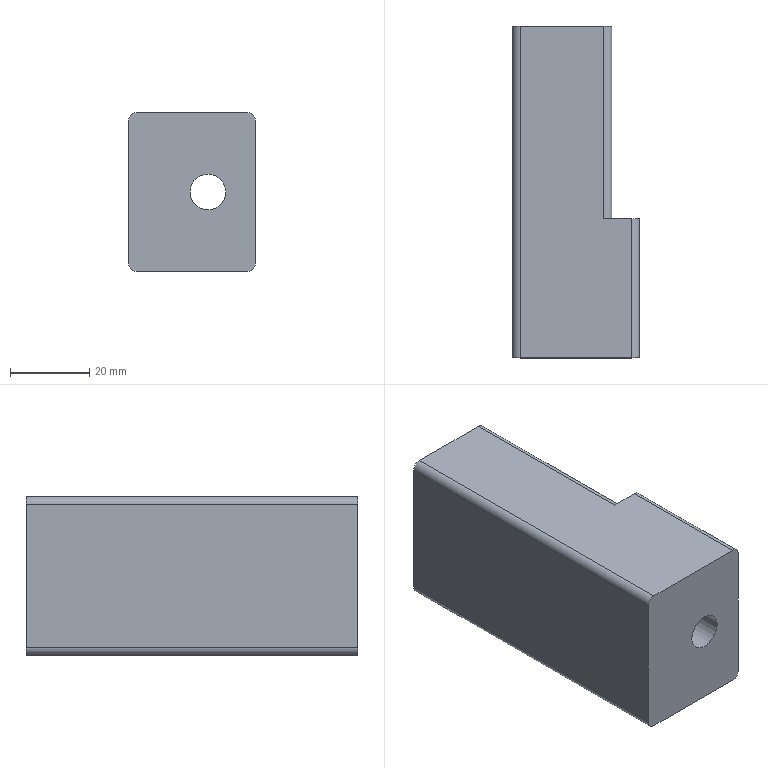NC program | Mastercam | posted with a generic post | part box 32 x 83.5 x 40 mm
Lines 3946 to 4494 of 4494:
(10 FEM |TOOL - 10|DIA. OFF. - 10|LEN. - 10|TOOL DIA. - 10.)
N7946 T10 M6
N7948 G0 G54 G90 X.341 Y-22.678 C0. B0. S7000 M3
N7950 G43 H10 Z50.
N7952 Z1.
N7954 G1 Z-9.7 F600.
N7956 X4.841 Y-5.25 F1000.
N7958 G3 X5. Y-4. I-4.841 J1.25
N7960 X0. Y1. I-5.
N7962 X-5. Y-4. J-5.
N7964 X-4.841 Y-5.25 I5.
N7966 G1 X-.341 Y-22.678
N7968 X.341
N7970 Z-19.4 F600.
N7972 X4.841 Y-5.25 F1000.
N7974 G3 X5. Y-4. I-4.841 J1.25
N7976 X0. Y1. I-5.
N7978 X-5. Y-4. J-5.
N7980 X-4.841 Y-5.25 I5.
N7982 G1 X-.341 Y-22.678
N7984 X.341
N7986 Z-29.1 F600.
N7988 X4.841 Y-5.25 F1000.
N7990 G3 X5. Y-4. I-4.841 J1.25
N7992 X0. Y1. I-5.
N7994 X-5. Y-4. J-5.
N7996 X-4.841 Y-5.25 I5.
N7998 G1 X-.341 Y-22.678
N8000 X.341
N8002 Z-38.8 F600.
N8004 X4.841 Y-5.25 F1000.
N8006 G3 X5. Y-4. I-4.841 J1.25
N8008 X0. Y1. I-5.
N8010 X-5. Y-4. J-5.
N8012 X-4.841 Y-5.25 I5.
N8014 G1 X-.341 Y-22.678
N8016 X.341
N8018 Z-48.5 F600.
N8020 X4.841 Y-5.25 F1000.
N8022 G3 X5. Y-4. I-4.841 J1.25
N8024 X0. Y1. I-5.
N8026 X-5. Y-4. J-5.
N8028 X-4.841 Y-5.25 I5.
N8030 G1 X-.341 Y-22.678
N8032 G0 Z50.
N8034 X27. Y-6.
N8036 Z1.
N8038 G1 Z-9.7 F600.
N8040 X26. F1000.
N8042 G3 X25. Y-7. J-1.
N8044 G2 X18. Y-14. I-7.
N8046 G1 X11.619
N8048 G2 X4.619 Y-7. J7.
N8050 X4.841 Y-5.25 I7.
N8052 G3 X5. Y-4. I-4.841 J1.25
N8054 X0. Y1. I-5.
N8056 X-5. Y-4. J-5.
N8058 X-4.841 Y-5.25 I5.
N8060 G2 X-4.619 Y-7. I-6.778 J-1.75
N8062 X-11.619 Y-14. I-7.
N8064 G1 X-18.
N8066 G2 X-25. Y-7. J7.
N8068 G3 X-26. Y-6. I-1.
N8070 G1 X-27.
N8072 G0 Z50.
N8074 X27.
N8076 Z-8.7
N8078 G1 Z-19.4 F600.
N8080 X26. F1000.
N8082 G3 X25. Y-7. J-1.
N8084 G2 X18. Y-14. I-7.
N8086 G1 X11.619
N8088 G2 X4.619 Y-7. J7.
N8090 X4.841 Y-5.25 I7.
N8092 G3 X5. Y-4. I-4.841 J1.25
N8094 X0. Y1. I-5.
N8096 X-5. Y-4. J-5.
N8098 X-4.841 Y-5.25 I5.
N8100 G2 X-4.619 Y-7. I-6.778 J-1.75
N8102 X-11.619 Y-14. I-7.
N8104 G1 X-18.
N8106 G2 X-25. Y-7. J7.
N8108 G3 X-26. Y-6. I-1.
N8110 G1 X-27.
N8112 G0 Z50.
N8114 X27.
N8116 Z-18.4
N8118 G1 Z-29.1 F600.
N8120 X26. F1000.
N8122 G3 X25. Y-7. J-1.
N8124 G2 X18. Y-14. I-7.
N8126 G1 X11.619
N8128 G2 X4.619 Y-7. J7.
N8130 X4.841 Y-5.25 I7.
N8132 G3 X5. Y-4. I-4.841 J1.25
N8134 X0. Y1. I-5.
N8136 X-5. Y-4. J-5.
N8138 X-4.841 Y-5.25 I5.
N8140 G2 X-4.619 Y-7. I-6.778 J-1.75
N8142 X-11.619 Y-14. I-7.
N8144 G1 X-18.
N8146 G2 X-25. Y-7. J7.
N8148 G3 X-26. Y-6. I-1.
N8150 G1 X-27.
N8152 G0 Z50.
N8154 X27.
N8156 Z-28.1
N8158 G1 Z-38.8 F600.
N8160 X26. F1000.
N8162 G3 X25. Y-7. J-1.
N8164 G2 X18. Y-14. I-7.
N8166 G1 X11.619
N8168 G2 X4.619 Y-7. J7.
N8170 X4.841 Y-5.25 I7.
N8172 G3 X5. Y-4. I-4.841 J1.25
N8174 X0. Y1. I-5.
N8176 X-5. Y-4. J-5.
N8178 X-4.841 Y-5.25 I5.
N8180 G2 X-4.619 Y-7. I-6.778 J-1.75
N8182 X-11.619 Y-14. I-7.
N8184 G1 X-18.
N8186 G2 X-25. Y-7. J7.
N8188 G3 X-26. Y-6. I-1.
N8190 G1 X-27.
N8192 G0 Z50.
N8194 X27.
N8196 Z-37.8
N8198 G1 Z-48.5 F600.
N8200 X26. F1000.
N8202 G3 X25. Y-7. J-1.
N8204 G2 X18. Y-14. I-7.
N8206 G1 X11.619
N8208 G2 X4.619 Y-7. J7.
N8210 X4.841 Y-5.25 I7.
N8212 G3 X5. Y-4. I-4.841 J1.25
N8214 X0. Y1. I-5.
N8216 X-5. Y-4. J-5.
N8218 X-4.841 Y-5.25 I5.
N8220 G2 X-4.619 Y-7. I-6.778 J-1.75
N8222 X-11.619 Y-14. I-7.
N8224 G1 X-18.
N8226 G2 X-25. Y-7. J7.
N8228 G3 X-26. Y-6. I-1.
N8230 G1 X-27.
N8232 G0 Z50.
N8234 M5
N8236 G0 G28 G91 Z0.
N8238 G28
N8240 M01
N8242 G0 G17 G40 G80 G90 G94 G98
N8244 G0 G28 G91 Z0.
(4 CHM |TOOL - 5|DIA. OFF. - 5|LEN. - 5|TOOL DIA. - 4.)
N8246 T5 M6
N8248 G0 G54 G90 X-18.4 Y17.45 C0. B0. S7000 M3
N8250 G43 H5 Z50.
N8252 Z1.
N8254 G1 Z-.75 F600.
N8256 Y17.05 F1000.
N8258 G3 X-18. Y16.65 I.4
N8260 G1 X18.
N8262 G2 X20.65 Y14. J-2.65
N8264 G1 Y-7.
N8266 G2 X18. Y-9.65 I-2.65
N8268 G1 X11.619
N8270 G2 X8.969 Y-7. J2.65
N8272 X9.053 Y-6.338 I2.65
N8274 G3 X9.35 Y-4. I-9.053 J2.338
N8276 X0. Y5.35 I-9.35
N8278 X-9.35 Y-4. J-9.35
N8280 X-9.053 Y-6.338 I9.35
N8282 G2 X-8.969 Y-7. I-2.566 J-.662
N8284 X-11.619 Y-9.65 I-2.65
N8286 G1 X-18.
N8288 G2 X-20.65 Y-7. J2.65
N8290 G1 Y14.
N8292 G2 X-18. Y16.65 I2.65
N8294 G3 X-17.6 Y17.05 J.4
N8296 G1 Y17.45
N8298 G0 Z50.
N8300 M5
N8302 G0 G28 G91 Z0.
N8304 G28
N8306 M01
N8308 G0 G17 G40 G80 G90 G94 G98
N8310 G0 G28 G91 Z0.
(12 FEM |TOOL - 12|DIA. OFF. - 12|LEN. - 12|TOOL DIA. - 12.)
N8312 T12 M6
N8314 G0 G54 G90 X.5 Y-2.8 C0. B0. S5000 M3
N8316 G43 H12 Z50.
N8318 Z-47.5
N8320 G1 Z-48.5 F600.
N8322 X-.7 F1000.
N8324 G3 X-1.9 Y-4. J-1.2
N8326 X0. Y-5.9 Z-48.55 I1.9
N8328 X1.9 Y-4. Z-48.6 J1.9
N8330 X0. Y-2.1 Z-48.65 I-1.9
N8332 X-1.9 Y-4. Z-48.7 J-1.9
N8334 X0. Y-5.9 Z-48.75 I1.9
N8336 X1.9 Y-4. Z-48.8 J1.9
N8338 X0. Y-2.1 Z-48.85 I-1.9
N8340 X-1.9 Y-4. Z-48.9 J-1.9
N8342 X0. Y-5.9 Z-48.95 I1.9
N8344 X1.9 Y-4. Z-49. J1.9
N8346 X0. Y-2.1 Z-49.05 I-1.9
N8348 X-1.9 Y-4. Z-49.1 J-1.9
N8350 X0. Y-5.9 Z-49.15 I1.9
N8352 X1.9 Y-4. Z-49.2 J1.9
N8354 X0. Y-2.1 Z-49.25 I-1.9
N8356 X-1.9 Y-4. Z-49.3 J-1.9
N8358 X0. Y-5.9 Z-49.35 I1.9
N8360 X1.9 Y-4. Z-49.4 J1.9
N8362 X0. Y-2.1 Z-49.45 I-1.9
N8364 X-1.9 Y-4. Z-49.5 J-1.9
N8366 X0. Y-5.9 Z-49.55 I1.9
N8368 X1.9 Y-4. Z-49.6 J1.9
N8370 X0. Y-2.1 Z-49.65 I-1.9
N8372 X-1.9 Y-4. Z-49.7 J-1.9
N8374 X0. Y-5.9 Z-49.75 I1.9
N8376 X1.9 Y-4. Z-49.8 J1.9
N8378 X0. Y-2.1 Z-49.85 I-1.9
N8380 X-1.9 Y-4. Z-49.9 J-1.9
N8382 X0. Y-5.9 Z-49.95 I1.9
N8384 X1.9 Y-4. Z-50. J1.9
N8386 X0. Y-2.1 Z-50.05 I-1.9
N8388 X-1.9 Y-4. Z-50.1 J-1.9
N8390 X0. Y-5.9 Z-50.15 I1.9
N8392 X1.9 Y-4. Z-50.2 J1.9
N8394 X0. Y-2.1 Z-50.25 I-1.9
N8396 X-1.9 Y-4. Z-50.3 J-1.9
N8398 X0. Y-5.9 Z-50.35 I1.9
N8400 X1.9 Y-4. Z-50.4 J1.9
N8402 X0. Y-2.1 Z-50.45 I-1.9
N8404 X-1.9 Y-4. Z-50.5 J-1.9
N8406 X0. Y-5.9 Z-50.55 I1.9
N8408 X1.9 Y-4. Z-50.6 J1.9
N8410 X0. Y-2.1 Z-50.65 I-1.9
N8412 X-1.9 Y-4. Z-50.7 J-1.9
N8414 X0. Y-5.9 Z-50.75 I1.9
N8416 X1.9 Y-4. Z-50.8 J1.9
N8418 X0. Y-2.1 Z-50.85 I-1.9
N8420 X-1.9 Y-4. Z-50.9 J-1.9
N8422 X0. Y-5.9 Z-50.95 I1.9
N8424 X1.9 Y-4. Z-51. J1.9
N8426 X0. Y-2.1 Z-51.05 I-1.9
N8428 X-1.9 Y-4. Z-51.1 J-1.9
N8430 X0. Y-5.9 Z-51.15 I1.9
N8432 X1.9 Y-4. Z-51.2 J1.9
N8434 X0. Y-2.1 Z-51.25 I-1.9
N8436 X-1.9 Y-4. Z-51.3 J-1.9
N8438 X0. Y-5.9 Z-51.35 I1.9
N8440 X1.9 Y-4. Z-51.4 J1.9
N8442 X0. Y-2.1 Z-51.45 I-1.9
N8444 X-1.9 Y-4. Z-51.5 J-1.9
N8446 X0. Y-5.9 Z-51.55 I1.9
N8448 X1.9 Y-4. Z-51.6 J1.9
N8450 X0. Y-2.1 Z-51.65 I-1.9
N8452 X-1.9 Y-4. Z-51.7 J-1.9
N8454 X0. Y-5.9 Z-51.75 I1.9
N8456 X1.9 Y-4. Z-51.8 J1.9
N8458 X0. Y-2.1 Z-51.85 I-1.9
N8460 X-1.9 Y-4. Z-51.9 J-1.9
N8462 X0. Y-5.9 Z-51.95 I1.9
N8464 X1.9 Y-4. Z-52. J1.9
N8466 X0. Y-2.1 Z-52.05 I-1.9
N8468 X-1.9 Y-4. Z-52.1 J-1.9
N8470 X0. Y-5.9 Z-52.15 I1.9
N8472 X1.9 Y-4. Z-52.2 J1.9
N8474 X0. Y-2.1 Z-52.25 I-1.9
N8476 X-1.9 Y-4. Z-52.3 J-1.9
N8478 X0. Y-5.9 Z-52.35 I1.9
N8480 X1.9 Y-4. Z-52.4 J1.9
N8482 X0. Y-2.1 Z-52.45 I-1.9
N8484 X-1.9 Y-4. Z-52.5 J-1.9
N8486 X0. Y-5.9 Z-52.55 I1.9
N8488 X1.9 Y-4. Z-52.6 J1.9
N8490 X0. Y-2.1 Z-52.65 I-1.9
N8492 X-1.9 Y-4. Z-52.7 J-1.9
N8494 X0. Y-5.9 Z-52.75 I1.9
N8496 X1.9 Y-4. Z-52.8 J1.9
N8498 X0. Y-2.1 Z-52.85 I-1.9
N8500 X-1.9 Y-4. Z-52.9 J-1.9
N8502 X0. Y-5.9 Z-52.95 I1.9
N8504 X1.9 Y-4. Z-53. J1.9
N8506 X0. Y-2.1 Z-53.05 I-1.9
N8508 X-1.9 Y-4. Z-53.1 J-1.9
N8510 X0. Y-5.9 Z-53.15 I1.9
N8512 X1.9 Y-4. Z-53.2 J1.9
N8514 X0. Y-2.1 Z-53.25 I-1.9
N8516 X-1.9 Y-4. Z-53.3 J-1.9
N8518 X0. Y-5.9 Z-53.35 I1.9
N8520 X1.9 Y-4. Z-53.4 J1.9
N8522 X0. Y-2.1 I-1.9
N8524 X-1.9 Y-4. J-1.9
N8526 X0. Y-5.9 I1.9
N8528 X1.9 Y-4. J1.9
N8530 X.7 Y-2.8 I-1.2
N8532 G1 X-.5
N8534 G0 Z50.
N8536 X-.8 Y-3.4
N8538 Z-47.5
N8540 G1 Z-53.5 F600.
N8542 X-1.4 F300.
N8544 G3 X-2. Y-4. J-.6
N8546 X0. Y-6. I2.
N8548 X2. Y-4. J2.
N8550 X0. Y-2. I-2.
N8552 X-2. Y-4. J-2.
N8554 X-1.4 Y-4.6 I.6
N8556 G1 X-.8
N8558 G0 Z50.
N8560 Y-3.4
N8562 Z-47.5
N8564 G1 Z-53.5 F600.
N8566 X-1.4 F300.
N8568 G3 X-2. Y-4. J-.6
N8570 X0. Y-6. I2.
N8572 X2. Y-4. J2.
N8574 X0. Y-2. I-2.
N8576 X-2. Y-4. J-2.
N8578 X-1.4 Y-4.6 I.6
N8580 G1 X-.8
N8582 G0 Z50.
N8584 M5
N8586 G0 G28 G91 Z0.
N8588 G28
N8590 M01
N8592 G0 G17 G40 G80 G90 G94 G98
N8594 G0 G28 G91 Z0.
(2 FEM |TOOL - 1|DIA. OFF. - 1|LEN. - 1|TOOL DIA. - 2.)
N8596 T1 M6
N8598 G0 G54 G90 X-7. Y-4. C0. B0. S3500 M3
N8600 G43 H1 Z50.
N8602 Z-52.5
N8604 G1 Z-53.5 F600.
N8606 G3 X0. Y-11. Z-53.512 I7. F500.
N8608 X7. Y-4. Z-53.525 J7.
N8610 X0. Y3. Z-53.537 I-7.
N8612 X-7. Y-4. Z-53.55 J-7.
N8614 X0. Y-11. Z-53.563 I7.
N8616 X7. Y-4. Z-53.575 J7.
N8618 X0. Y3. Z-53.587 I-7.
N8620 X-7. Y-4. Z-53.6 J-7.
N8622 X0. Y-11. Z-53.612 I7.
N8624 X7. Y-4. Z-53.625 J7.
N8626 X0. Y3. Z-53.637 I-7.
N8628 X-7. Y-4. Z-53.65 J-7.
N8630 X0. Y-11. Z-53.663 I7.
N8632 X7. Y-4. Z-53.675 J7.
N8634 X0. Y3. Z-53.688 I-7.
N8636 X-7. Y-4. Z-53.7 J-7.
N8638 X0. Y-11. Z-53.712 I7.
N8640 X7. Y-4. Z-53.725 J7.
N8642 X0. Y3. Z-53.737 I-7.
N8644 X-7. Y-4. Z-53.75 J-7.
N8646 X0. Y-11. Z-53.762 I7.
N8648 X7. Y-4. Z-53.775 J7.
N8650 X0. Y3. Z-53.787 I-7.
N8652 X-7. Y-4. Z-53.8 J-7.
N8654 X0. Y-11. Z-53.813 I7.
N8656 X7. Y-4. Z-53.825 J7.
N8658 X0. Y3. Z-53.837 I-7.
N8660 X-7. Y-4. Z-53.85 J-7.
N8662 X0. Y-11. Z-53.862 I7.
N8664 X7. Y-4. Z-53.875 J7.
N8666 X0. Y3. Z-53.887 I-7.
N8668 X-7. Y-4. Z-53.9 J-7.
N8670 X0. Y-11. Z-53.913 I7.
N8672 X7. Y-4. Z-53.925 J7.
N8674 X0. Y3. Z-53.938 I-7.
N8676 X-7. Y-4. Z-53.95 J-7.
N8678 X0. Y-11. Z-53.962 I7.
N8680 X7. Y-4. Z-53.975 J7.
N8682 X0. Y3. Z-53.987 I-7.
N8684 X-7. Y-4. Z-54. J-7.
N8686 X0. Y-11. Z-54.012 I7.
N8688 X7. Y-4. Z-54.025 J7.
N8690 X0. Y3. Z-54.037 I-7.
N8692 X-7. Y-4. Z-54.05 J-7.
N8694 X0. Y-11. Z-54.063 I7.
N8696 X7. Y-4. Z-54.075 J7.
N8698 X0. Y3. Z-54.087 I-7.
N8700 X-7. Y-4. Z-54.1 J-7.
N8702 X0. Y-11. Z-54.112 I7.
N8704 X7. Y-4. Z-54.125 J7.
N8706 X0. Y3. Z-54.137 I-7.
N8708 X-7. Y-4. Z-54.15 J-7.
N8710 X0. Y-11. Z-54.163 I7.
N8712 X7. Y-4. Z-54.175 J7.
N8714 X0. Y3. Z-54.188 I-7.
N8716 X-7. Y-4. Z-54.2 J-7.
N8718 X0. Y-11. Z-54.212 I7.
N8720 X7. Y-4. Z-54.225 J7.
N8722 X0. Y3. Z-54.237 I-7.
N8724 X-7. Y-4. Z-54.25 J-7.
N8726 X0. Y-11. Z-54.262 I7.
N8728 X7. Y-4. Z-54.275 J7.
N8730 X0. Y3. Z-54.287 I-7.
N8732 X-7. Y-4. Z-54.3 J-7.
N8734 X0. Y-11. Z-54.313 I7.
N8736 X7. Y-4. Z-54.325 J7.
N8738 X0. Y3. Z-54.337 I-7.
N8740 X-7. Y-4. Z-54.35 J-7.
N8742 X0. Y-11. Z-54.362 I7.
N8744 X7. Y-4. Z-54.375 J7.
N8746 X0. Y3. Z-54.387 I-7.
N8748 X-7. Y-4. Z-54.4 J-7.
N8750 X0. Y-11. Z-54.413 I7.
N8752 X7. Y-4. Z-54.425 J7.
N8754 X0. Y3. Z-54.438 I-7.
N8756 X-7. Y-4. Z-54.45 J-7.
N8758 X0. Y-11. Z-54.462 I7.
N8760 X7. Y-4. Z-54.475 J7.
N8762 X0. Y3. Z-54.487 I-7.
N8764 X-7. Y-4. Z-54.5 J-7.
N8766 X0. Y-11. Z-54.512 I7.
N8768 X7. Y-4. Z-54.525 J7.
N8770 X0. Y3. Z-54.537 I-7.
N8772 X-7. Y-4. Z-54.55 J-7.
N8774 X0. Y-11. Z-54.563 I7.
N8776 X7. Y-4. Z-54.575 J7.
N8778 X0. Y3. Z-54.587 I-7.
N8780 X-7. Y-4. Z-54.6 J-7.
N8782 X0. Y-11. Z-54.612 I7.
N8784 X7. Y-4. Z-54.625 J7.
N8786 X0. Y3. Z-54.637 I-7.
N8788 X-7. Y-4. Z-54.65 J-7.
N8790 X0. Y-11. Z-54.663 I7.
N8792 X7. Y-4. Z-54.675 J7.
N8794 X0. Y3. Z-54.688 I-7.
N8796 X-7. Y-4. Z-54.7 J-7.
N8798 X0. Y-11. Z-54.712 I7.
N8800 X7. Y-4. Z-54.725 J7.
N8802 X0. Y3. Z-54.737 I-7.
N8804 X-7. Y-4. Z-54.75 J-7.
N8806 X0. Y-11. Z-54.762 I7.
N8808 X7. Y-4. Z-54.775 J7.
N8810 X0. Y3. Z-54.787 I-7.
N8812 X-7. Y-4. Z-54.8 J-7.
N8814 X0. Y-11. Z-54.813 I7.
N8816 X7. Y-4. Z-54.825 J7.
N8818 X0. Y3. Z-54.837 I-7.
N8820 X-7. Y-4. Z-54.85 J-7.
N8822 X0. Y-11. Z-54.862 I7.
N8824 X7. Y-4. Z-54.875 J7.
N8826 X0. Y3. Z-54.887 I-7.
N8828 X-7. Y-4. Z-54.9 J-7.
N8830 X0. Y-11. Z-54.913 I7.
N8832 X7. Y-4. Z-54.925 J7.
N8834 X0. Y3. Z-54.938 I-7.
N8836 X-7. Y-4. Z-54.95 J-7.
N8838 X0. Y-11. Z-54.962 I7.
N8840 X7. Y-4. Z-54.975 J7.
N8842 X0. Y3. Z-54.987 I-7.
N8844 X-7. Y-4. Z-55. J-7.
N8846 X0. Y-11. Z-55.012 I7.
N8848 X7. Y-4. Z-55.025 J7.
N8850 X0. Y3. Z-55.037 I-7.
N8852 X-7. Y-4. Z-55.05 J-7.
N8854 X0. Y-11. Z-55.063 I7.
N8856 X7. Y-4. Z-55.075 J7.
N8858 X0. Y3. Z-55.087 I-7.
N8860 X-7. Y-4. Z-55.1 J-7.
N8862 X0. Y-11. Z-55.112 I7.
N8864 X7. Y-4. Z-55.125 J7.
N8866 X0. Y3. Z-55.137 I-7.
N8868 X-7. Y-4. Z-55.15 J-7.
N8870 X0. Y-11. Z-55.163 I7.
N8872 X7. Y-4. Z-55.175 J7.
N8874 X0. Y3. Z-55.188 I-7.
N8876 X-7. Y-4. Z-55.2 J-7.
N8878 X0. Y-11. Z-55.212 I7.
N8880 X7. Y-4. Z-55.225 J7.
N8882 X0. Y3. Z-55.237 I-7.
N8884 X-7. Y-4. Z-55.25 J-7.
N8886 X0. Y-11. Z-55.262 I7.
N8888 X7. Y-4. Z-55.275 J7.
N8890 X0. Y3. Z-55.287 I-7.
N8892 X-7. Y-4. Z-55.3 J-7.
N8894 X0. Y-11. Z-55.313 I7.
N8896 X7. Y-4. Z-55.325 J7.
N8898 X0. Y3. Z-55.337 I-7.
N8900 X-7. Y-4. Z-55.35 J-7.
N8902 X0. Y-11. Z-55.362 I7.
N8904 X7. Y-4. Z-55.375 J7.
N8906 X0. Y3. Z-55.387 I-7.
N8908 X-7. Y-4. Z-55.4 J-7.
N8910 X0. Y-11. Z-55.413 I7.
N8912 X7. Y-4. Z-55.425 J7.
N8914 X0. Y3. Z-55.438 I-7.
N8916 X-7. Y-4. Z-55.45 J-7.
N8918 X0. Y-11. Z-55.462 I7.
N8920 X7. Y-4. Z-55.475 J7.
N8922 X0. Y3. Z-55.487 I-7.
N8924 X-7. Y-4. Z-55.5 J-7.
N8926 X0. Y-11. I7.
N8928 X7. Y-4. J7.
N8930 X0. Y3. I-7.
N8932 X-7. Y-4. J-7.
N8934 G0 Z50.
N8936 M5
N8938 G0 G28 G91 Z0.
N8940 G28
N8942 M01
N8944 G0 G17 G40 G80 G90 G94 G98
N8946 G0 G28 G91 Z0.
(6 CHM |TOOL - 7|DIA. OFF. - 7|LEN. - 7|TOOL DIA. - 6.)
N8948 T7 M6
N8950 G0 G54 G90 X22.65 Y-10.913 C0. B0. S5000 M3
N8952 G43 H7 Z24.689
N8954 Z-15.2
N8956 Z-40.2
N8958 G1 Z-50.2 F600.
N8960 X22.15 F500.
N8962 G3 X21.65 Y-11.413 J-.5
N8964 G1 Y-14.
N8966 G2 X18. Y-17.65 I-3.65
N8968 G1 X-18.
N8970 G2 X-21.65 Y-14. J3.65
N8972 G1 Y-11.413
N8974 G3 X-22.15 Y-10.913 I-.5
N8976 G1 X-22.65
N8978 G0 Z-25.2
N8980 Z25.
N8982 X-14. Y-7.207
N8984 X-5.35 Y-3.5
N8986 Z-15.2
N8988 Z-40.2
N8990 G1 Z-50.2 F600.
N8992 X-5.85 F500.
N8994 G3 X-6.35 Y-4. J-.5
N8996 X0. Y-10.35 I6.35
N8998 X6.35 Y-4. J6.35
N9000 X0. Y2.35 I-6.35
N9002 X-6.35 Y-4. J-6.35
N9004 X-5.85 Y-4.5 I.5
N9006 G1 X-5.35
N9008 G0 Z-25.2
N9010 Z24.596
N9012 S3000 M3
N9014 Z46.5
N9016 X0. Y-4.
N9018 G81 G98 Z-54.2 R-52.5 F300.
N9020 G80
N9022 M5
N9024 G0 G28 G91 Z0.
N9026 G0 G28 X0. Y0.
N9028 G28
N9030 M30
%